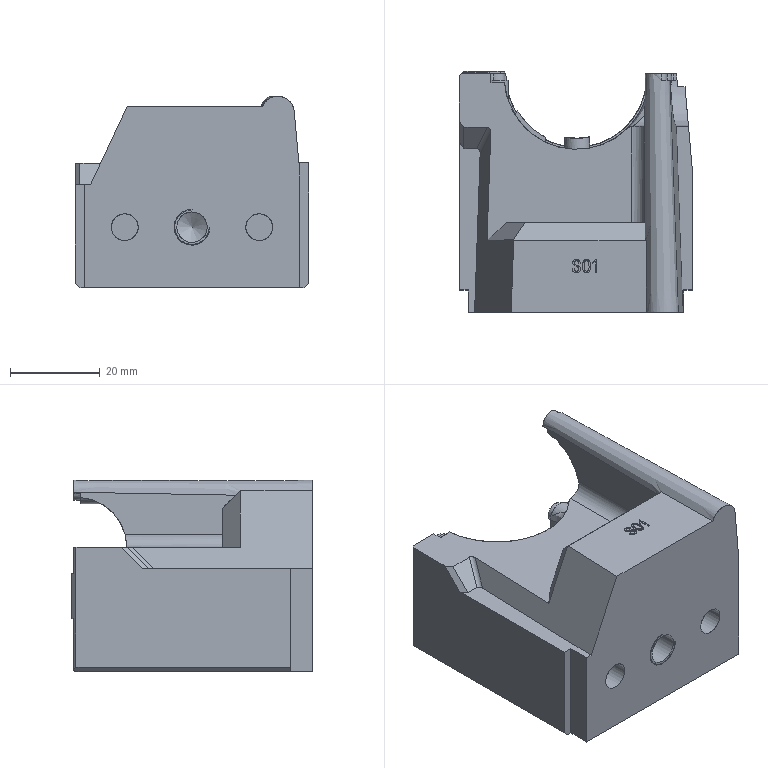CAM job | PowerMill | 3+2 milling, other | part box 52 x 53.756 x 42.711 mm | stock box 52 x 53.756 x 44.71 mm
Tools:
number,name,type,diameter,tip_radius,length,cutting_length,overhang,flutes,holder,toolpaths_using
0,D6_3,end_mill,6.0,0.0,50.0,,6.0,1,D35L68,3
0,D8_3,end_mill,8.0,0.0,60.0,,8.0,1,D35L68,2
0,D8_2,end_mill,8.0,0.0,60.0,,8.0,1,D35L68,1
0,D8_1,end_mill,8.0,0.0,60.0,,8.0,1,D35L68,1
0,B13R0.8,tip_radiused,13.0,0.8,50.0,,30.0,1,D50L68,1
0,B13R0.8_1_1,tip_radiused,13.0,0.8,50.0,,23.16,1,D50L68,1
0,D6_1_1,end_mill,6.0,0.0,50.0,,23.16,1,D35L68,1
0,D6_2_1,end_mill,6.0,0.0,50.0,,22.48,1,D35L68,3
0,R3_1_1_1,ball_nosed,6.0,3.0,30.0,,18.48,1,D35L68,2
0,R3_2_1_1_1,ball_nosed,6.0,3.0,30.0,,25.4,1,D35L68,3
0,D10_1_1,end_mill,10.0,0.0,75.0,,17.76,1,D50L68,1
0,D4_1_1,end_mill,4.0,0.0,30.0,,17.56,1,D35L68,2
0,D8_4_1,end_mill,8.0,0.0,60.0,,17.76,1,D35L68,3
0,R2_1_1,ball_nosed,4.0,2.0,30.0,,5.6,1,D35L68,1
0,B8R0.5_1_1,tip_radiused,8.0,0.5,50.0,,17.76,1,D35L68,1
0,D4_3_1,end_mill,4.0,0.0,30.0,,17.72,1,D35L68,1
0,D2_1_1,end_mill,2.0,0.0,3.0,,15.32,1,D35L68,1
Operations:
program,toolpath,strategy,tool,tool_number,tool_diameter,tip_radius,flutes,spindle_rpm,feed_cut,surface_speed_m_min_computed,feed_per_tooth_computed,tolerance,thickness,stepover,stepdown,cut_length,cut_time_min,total_time_min,workplane
04-S01-0420A-1,01开粗-D8-等高,constantz,D8_1,0,8.0,0.0,1.0,3500.0,3500.0,87.96,1.0,0.01,0.2,5.0,0.15,2818.86,0.805,1.038,1
04-S01-0420A-2,02开粗-D8-等高,constantz,D8_2,0,8.0,0.0,1.0,3500.0,2800.0,87.96,0.8,0.01,0.03,5.0,0.12,3474.593,1.241,1.593,1
04-S01-0420A-3,04精光-D8-偏置平坦面,offset_area_clear,D8_3,0,8.0,0.0,1.0,3500.0,800.0,87.96,0.2286,0.01,0.2,4.0,1.0,103.002,0.129,0.2264,1
04-S01-0420A-3,03精光-D8-等高,constantz,D8_3,0,8.0,0.0,1.0,5500.0,2000.0,138.23,0.3636,0.005,-0.01,5.0,0.1,4261.606,2.131,2.24,1
04-S01-0420B-1,05开粗-B13R0.8-偏置区域清除,offset_area_clear,B13R0.8_1_1,0,13.0,0.8,1.0,2200.0,4000.0,89.85,1.818,0.01,0.25,7.0,1.0,54203.093,13.551,17.866,2
04-S01-0420B-2,06开粗-D6-偏置区域二粗,offset_area_clear,D6_1_1,0,6.0,0.0,1.0,3800.0,4000.0,71.63,1.053,0.01,0.26,4.0,1.0,3966.572,0.992,2.894,2
04-S01-0420B-3,07中光-D6-偏置平坦面,offset_area_clear,D6_2_1,0,6.0,0.0,1.0,5000.0,1200.0,94.25,0.24,0.01,0.5,3.0,1.0,336.424,0.28,0.4197,2
04-S01-0420B-3,08中光-D6-等高,constantz,D6_2_1,0,6.0,0.0,1.0,3800.0,3000.0,71.63,0.7895,0.01,0.05,5.0,0.1,100.736,0.034,0.0481,2
04-S01-0420B-3,25中光-D6-等高,constantz,D6_2_1,0,6.0,0.0,1.0,3800.0,3000.0,71.63,0.7895,0.01,0.05,5.0,0.1,5571.445,1.857,1.975,2
04-S01-0420B-4,09中光-R3-平行-已选面,raster,R3_1_1_1,0,6.0,3.0,1.0,5500.0,4000.0,103.67,0.7273,0.01,0.05,0.15,1.0,302.079,0.075,0.0921,2
04-S01-0420B-4,10中光-R3-最佳等高,opti_constz,R3_1_1_1,0,6.0,3.0,1.0,5500.0,4000.0,103.67,0.7273,0.01,0.05,0.1,1.0,3091.065,0.773,1.006,2
04-S01-0420B-5,13精光-D6-偏置平坦面,offset_area_clear,D6_3,0,6.0,0.0,1.0,6500.0,500.0,122.52,0.0769,0.01,0.3,3.0,1.0,253.132,0.506,0.6611,2
04-S01-0420B-5,14精光-D6-等高,constantz,D6_3,0,6.0,0.0,1.0,6500.0,2500.0,122.52,0.3846,0.005,0.0,5.0,0.05,131.396,0.053,0.0739,2
04-S01-0420B-5,26精光-D6-等高,constantz,D6_3,0,6.0,0.0,1.0,6500.0,2500.0,122.52,0.3846,0.005,0.0,5.0,0.05,862.21,0.345,0.4094,2
04-S01-0420B-6,11精光-R3-平行-已选面,raster,R3_2_1_1_1,0,6.0,3.0,1.0,6500.0,2200.0,122.52,0.3385,0.005,0.0,0.07,1.0,576.001,0.262,0.2821,2
04-S01-0420B-6,12精光-R3-最佳等高,opti_constz,R3_2_1_1_1,0,6.0,3.0,1.0,6500.0,2200.0,122.52,0.3385,0.005,0.0,0.07,1.0,2261.702,1.028,1.55,2
04-S01-0420B-6,16精光-R3-等高-已选面,constantz,R3_2_1_1_1,0,6.0,3.0,1.0,6500.0,2200.0,122.52,0.3385,0.005,-0.02,5.0,0.07,7764.101,3.529,4.033,2
04-S01-0420C-1,17开粗-D10-偏置区域二粗-残留模型,offset_area_clear,D10_1_1,0,10.0,0.0,1.0,3200.0,4000.0,100.53,1.25,0.02,0.2,6.0,1.0,27455.873,6.864,9.129,3
04-S01-0420C-2,18开粗-D4-等高,constantz,D4_1_1,0,4.0,0.0,1.0,5500.0,3000.0,69.12,0.5455,0.02,0.22,5.0,0.1,1257.097,0.419,0.5008,3
04-S01-0420C-3,19中光-D8-偏置平坦面,offset_area_clear,D8_4_1,0,8.0,0.0,1.0,5000.0,1200.0,125.66,0.24,0.02,0.5,4.0,1.0,506.188,0.422,0.5426,3
04-S01-0420C-3,20中光-D8-等高,constantz,D8_4_1,0,8.0,0.0,1.0,3500.0,3500.0,87.96,1.0,0.01,0.06,5.0,0.06,32384.535,9.253,9.841,3
04-S01-0420C-4,27中光-D4-等高-残留,constantz,D4_1_1,0,4.0,0.0,1.0,6500.0,4000.0,81.68,0.6154,0.01,0.06,5.0,0.07,1815.848,0.454,0.5332,3
04-S01-0420C-5,21精光-D8-偏置平坦面,offset_area_clear,D8_4_1,0,8.0,0.0,1.0,3500.0,800.0,87.96,0.2286,0.01,0.3,4.0,1.0,506.631,0.633,0.7943,3
04-S01-0420C-6,22精光-R2-平行-已选面,raster,R2_1_1,0,4.0,2.0,1.0,7000.0,1800.0,87.96,0.2571,0.005,0.0,0.06,1.0,10876.156,6.042,6.095,3
04-S01-0420C-7,23精光-B8R0.5-等高-已选面,constantz,B8R0.5_1_1,0,8.0,0.5,1.0,6000.0,2200.0,150.8,0.3667,0.005,0.0,5.0,0.04,27967.584,12.713,13.832,3
04-S01-0420C-8,24精光-D4-等高-残留,constantz,D4_3_1,0,4.0,0.0,1.0,6500.0,2000.0,81.68,0.3077,0.005,0.0,5.0,0.05,4063.834,2.032,2.254,3
04-S01-0420C-9,28精光-D2-等高-残留,constantz,D2_1_1,0,2.0,0.0,1.0,7500.0,2000.0,47.12,0.2667,0.005,0.0,5.0,0.02,1285.401,0.643,0.7078,3
,05开粗-B13R0.8-偏置区域清除_Reference,offset_area_clear,B13R0.8,0,13.0,0.8,1.0,2200.0,4000.0,89.85,1.818,0.01,0.25,7.0,1.0,72179.641,18.045,24.819,2